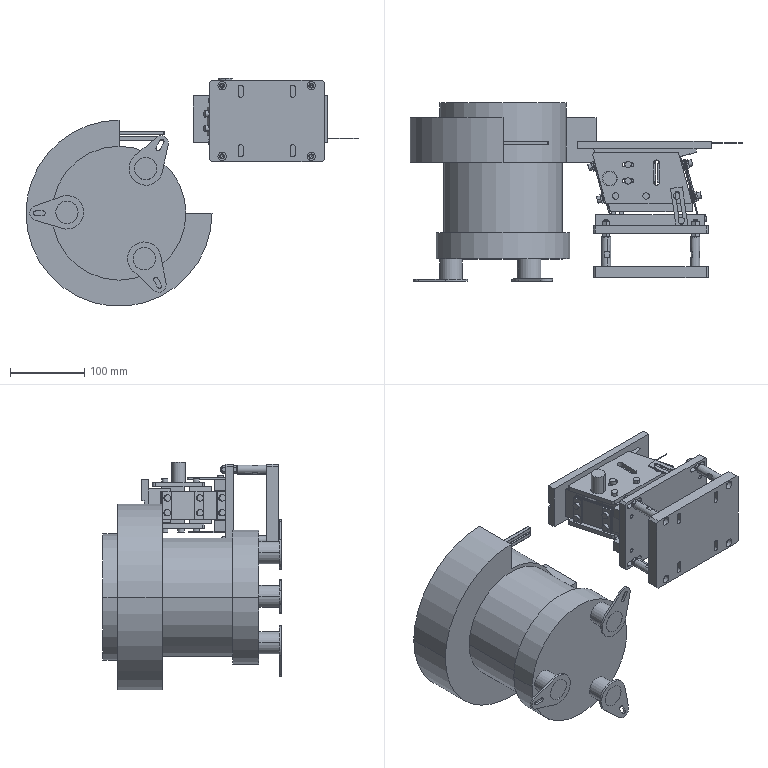Part | SolidWorks | 100 solids | 2027 faces | box 446.235 x 240 x 306.436 mm | volume 7009684 mm3 | plane 1334 | cylinder 538 | cone 155 | commonest cylinder face diameters 6 x121 4.2 x68 5 x68 5.4 x66 8.5 x52 2 x30